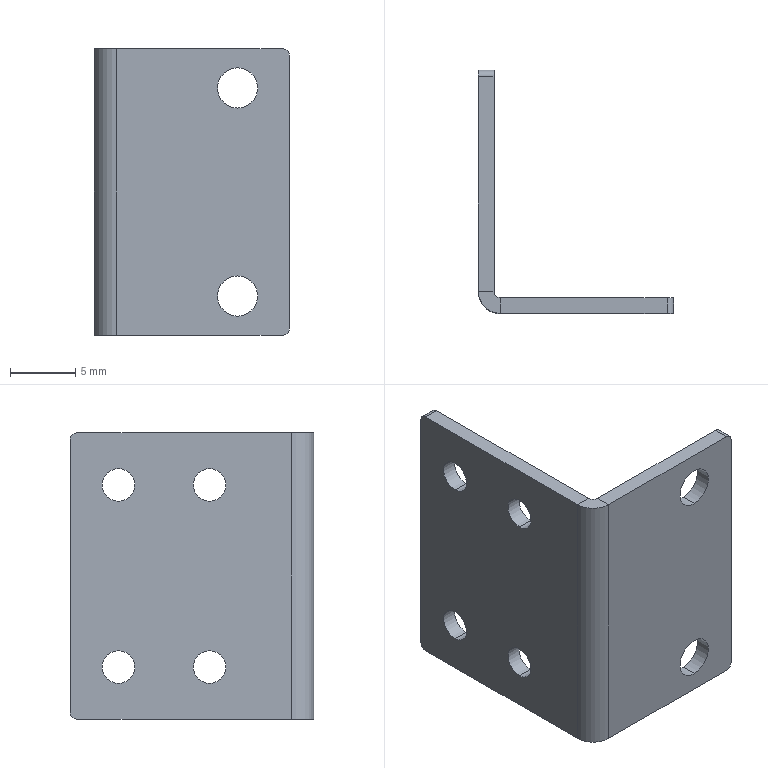Part | STEP file | 1 solid | 30 faces | box 15 x 18.7 x 22 mm | volume 803.602 mm3 | cylinder 18 | plane 12 | commonest cylinder face diameters 2.5 x8 1 x5 3.1 x4 3.4 x1